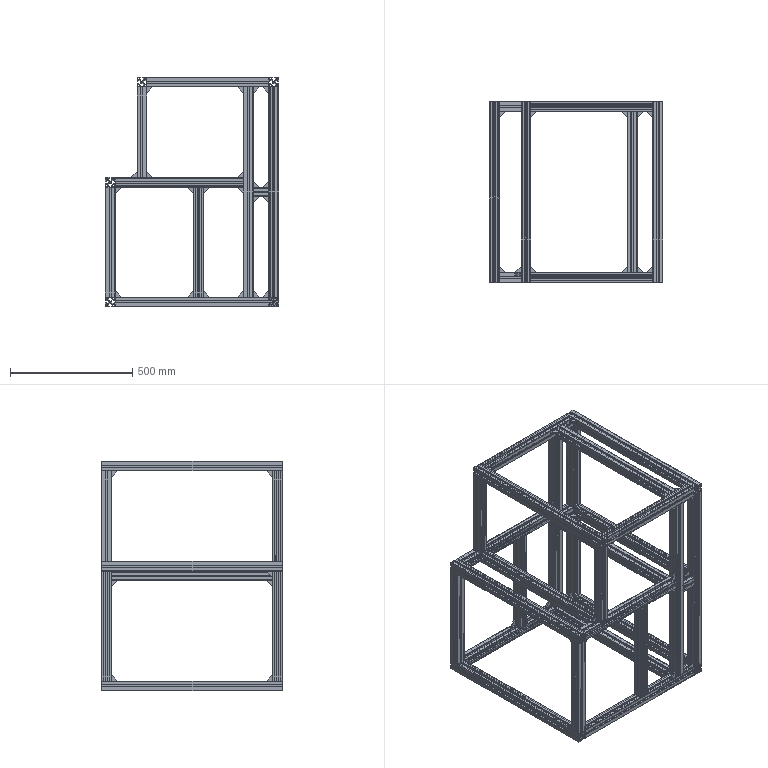Part | SolidWorks | features Gusset 71, WeldCornerFeat 9, 3DProfileFeature 1, WeldMemberFeat 1, WeldmentFeature 1 | 101 solids | 2035 faces | box 710 x 740 x 940 mm | volume 13346317 mm3 | plane 1615 | cylinder 420 | commonest cylinder face diameters 8 x240 1 x120 6.8 x60